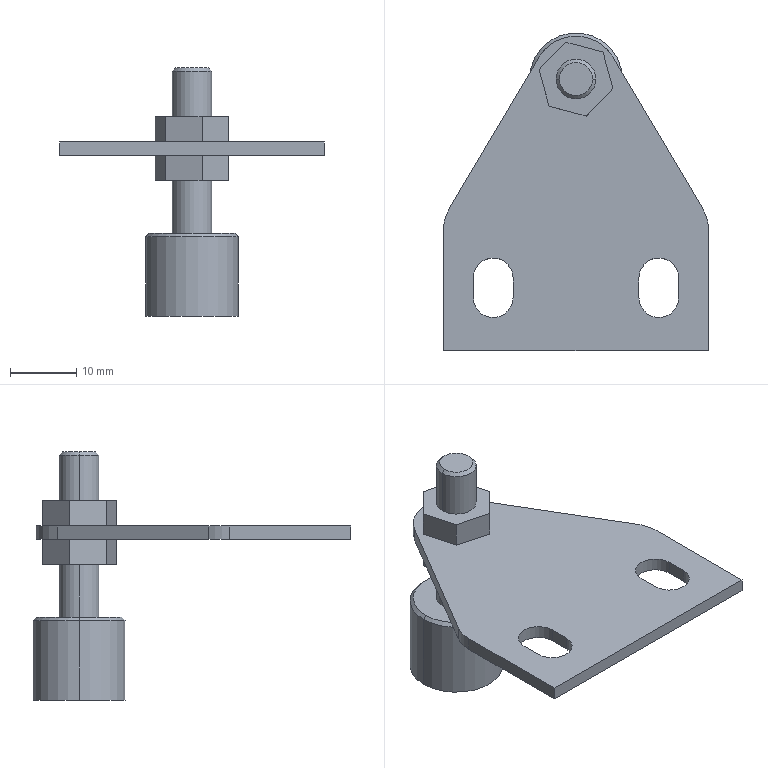Part | SolidWorks | features BaseBody 2 | 2 solids | 51 faces | box 40 x 48 x 37.5 mm | volume 5719 mm3 | plane 30 | cylinder 17 | cone 4 | commonest cylinder face diameters 6 x12 12 x2 14 x2 13 x1
STEP:
#1=CARTESIAN_POINT('',(-3.,41.,2.));
#2=VERTEX_POINT('',#1);
#3=CARTESIAN_POINT('',(3.,41.,2.));
#4=VERTEX_POINT('',#3);
#5=CARTESIAN_POINT('',(0.,41.,2.));
#6=DIRECTION('',(0.,0.,1.));
#7=DIRECTION('',(1.,0.,0.));
#8=AXIS2_PLACEMENT_3D('',#5,#6,#7);
#9=CIRCLE('',#8,3.);
#10=EDGE_CURVE('',#2,#4,#9,.T.);
#11=ORIENTED_EDGE('',*,*,#10,.T.);
#12=CARTESIAN_POINT('',(3.,41.,0.));
#13=VERTEX_POINT('',#12);
#14=CARTESIAN_POINT('',(3.,41.,2.));
#15=DIRECTION('',(0.,0.,-1.));
#16=VECTOR('',#15,1000.);
#17=LINE('',#14,#16);
#18=EDGE_CURVE('',#4,#13,#17,.T.);
#19=ORIENTED_EDGE('',*,*,#18,.T.);
#20=CARTESIAN_POINT('',(-3.,41.,0.));
#21=VERTEX_POINT('',#20);
#22=CARTESIAN_POINT('',(0.,41.,0.));
#23=DIRECTION('',(0.,0.,1.));
#24=DIRECTION('',(1.,0.,0.));
#25=AXIS2_PLACEMENT_3D('',#22,#23,#24);
#26=CIRCLE('',#25,3.);
#27=EDGE_CURVE('',#21,#13,#26,.T.);
#28=ORIENTED_EDGE('',*,*,#27,.F.);
#29=CARTESIAN_POINT('',(-3.,41.,2.));
#30=DIRECTION('',(0.,0.,-1.));
#31=VECTOR('',#30,1000.);
#32=LINE('',#29,#31);
#33=EDGE_CURVE('',#2,#21,#32,.T.);
#34=ORIENTED_EDGE('',*,*,#33,.F.);
#35=EDGE_LOOP('',(#11,#19,#28,#34));
#36=FACE_OUTER_BOUND('',#35,.T.);
#37=CARTESIAN_POINT('',(0.,41.,2.));
#38=DIRECTION('',(0.,0.,-1.));
#39=DIRECTION('',(-1.,0.,0.));
#40=AXIS2_PLACEMENT_3D('',#37,#38,#39);
#41=CYLINDRICAL_SURFACE('',#40,3.);
#42=ADVANCED_FACE('',(#36),#41,.F.);
#43=CARTESIAN_POINT('',(-9.5,11.,2.));
#44=VERTEX_POINT('',#43);
#45=CARTESIAN_POINT('',(-15.5,11.,2.));
#46=VERTEX_POINT('',#45);
#47=CARTESIAN_POINT('',(-12.5,11.,2.));
#48=DIRECTION('',(0.,0.,1.));
#49=DIRECTION('',(1.,0.,0.));
#50=AXIS2_PLACEMENT_3D('',#47,#48,#49);
#51=CIRCLE('',#50,3.);
#52=EDGE_CURVE('',#44,#46,#51,.T.);
#53=ORIENTED_EDGE('',*,*,#52,.F.);
#54=CARTESIAN_POINT('',(-9.5,8.,2.));
#55=VERTEX_POINT('',#54);
#56=CARTESIAN_POINT('',(-9.5,11.,2.));
#57=DIRECTION('',(0.,1.,0.));
#58=VECTOR('',#57,1000.);
#59=LINE('',#56,#58);
#60=EDGE_CURVE('',#55,#44,#59,.T.);
#61=ORIENTED_EDGE('',*,*,#60,.F.);
#62=CARTESIAN_POINT('',(-15.5,8.,2.));
#63=VERTEX_POINT('',#62);
#64=CARTESIAN_POINT('',(-12.5,8.,2.));
#65=DIRECTION('',(0.,0.,1.));
#66=DIRECTION('',(1.,0.,0.));
#67=AXIS2_PLACEMENT_3D('',#64,#65,#66);
#68=CIRCLE('',#67,3.);
#69=EDGE_CURVE('',#63,#55,#68,.T.);
#70=ORIENTED_EDGE('',*,*,#69,.F.);
#71=CARTESIAN_POINT('',(-15.5,11.,2.));
#72=DIRECTION('',(0.,-1.,0.));
#73=VECTOR('',#72,1000.);
#74=LINE('',#71,#73);
#75=EDGE_CURVE('',#46,#63,#74,.T.);
#76=ORIENTED_EDGE('',*,*,#75,.F.);
#77=EDGE_LOOP('',(#53,#61,#70,#76));
#78=FACE_BOUND('',#77,.T.);
#79=CARTESIAN_POINT('',(-20.,18.356,2.));
#80=VERTEX_POINT('',#79);
#81=CARTESIAN_POINT('',(-20.,0.,2.));
#82=VERTEX_POINT('',#81);
#83=CARTESIAN_POINT('',(-20.,0.,2.));
#84=DIRECTION('',(0.,-1.,0.));
#85=VECTOR('',#84,1000.);
#86=LINE('',#83,#85);
#87=EDGE_CURVE('',#80,#82,#86,.T.);
#88=ORIENTED_EDGE('',*,*,#87,.T.);
#89=CARTESIAN_POINT('',(20.,0.,2.));
#90=VERTEX_POINT('',#89);
#91=CARTESIAN_POINT('',(-20.,0.,2.));
#92=DIRECTION('',(1.,0.,0.));
#93=VECTOR('',#92,1000.);
#94=LINE('',#91,#93);
#95=EDGE_CURVE('',#82,#90,#94,.T.);
#96=ORIENTED_EDGE('',*,*,#95,.T.);
#97=CARTESIAN_POINT('',(20.,18.356,2.));
#98=VERTEX_POINT('',#97);
#99=CARTESIAN_POINT('',(20.,0.,2.));
#100=DIRECTION('',(0.,1.,0.));
#101=VECTOR('',#100,1000.);
#102=LINE('',#99,#101);
#103=EDGE_CURVE('',#90,#98,#102,.T.);
#104=ORIENTED_EDGE('',*,*,#103,.T.);
#105=CARTESIAN_POINT('',(19.162,21.415,2.));
#106=VERTEX_POINT('',#105);
#107=CARTESIAN_POINT('',(14.,18.356,2.));
#108=DIRECTION('',(0.,0.,1.));
#109=DIRECTION('',(-1.,0.,0.));
#110=AXIS2_PLACEMENT_3D('',#107,#108,#109);
#111=CIRCLE('',#110,6.);
#112=EDGE_CURVE('',#98,#106,#111,.T.);
#113=ORIENTED_EDGE('',*,*,#112,.T.);
#114=CARTESIAN_POINT('',(5.592,44.314,2.));
#115=VERTEX_POINT('',#114);
#116=CARTESIAN_POINT('',(19.162,21.415,2.));
#117=DIRECTION('',(-0.5098,0.8603,0.));
#118=VECTOR('',#117,1000.);
#119=LINE('',#116,#118);
#120=EDGE_CURVE('',#106,#115,#119,.T.);
#121=ORIENTED_EDGE('',*,*,#120,.T.);
#122=CARTESIAN_POINT('',(-5.592,44.314,2.));
#123=VERTEX_POINT('',#122);
#124=CARTESIAN_POINT('',(0.,41.,2.));
#125=DIRECTION('',(0.,0.,1.));
#126=DIRECTION('',(1.,0.,0.));
#127=AXIS2_PLACEMENT_3D('',#124,#125,#126);
#128=CIRCLE('',#127,6.5);
#129=EDGE_CURVE('',#115,#123,#128,.T.);
#130=ORIENTED_EDGE('',*,*,#129,.T.);
#131=CARTESIAN_POINT('',(-19.162,21.415,2.));
#132=VERTEX_POINT('',#131);
#133=CARTESIAN_POINT('',(-19.162,21.415,2.));
#134=DIRECTION('',(-0.5098,-0.8603,0.));
#135=VECTOR('',#134,1000.);
#136=LINE('',#133,#135);
#137=EDGE_CURVE('',#123,#132,#136,.T.);
#138=ORIENTED_EDGE('',*,*,#137,.T.);
#139=CARTESIAN_POINT('',(-14.,18.356,2.));
#140=DIRECTION('',(0.,0.,1.));
#141=DIRECTION('',(-1.,0.,0.));
#142=AXIS2_PLACEMENT_3D('',#139,#140,#141);
#143=CIRCLE('',#142,6.);
#144=EDGE_CURVE('',#132,#80,#143,.T.);
#145=ORIENTED_EDGE('',*,*,#144,.T.);
#146=EDGE_LOOP('',(#88,#96,#104,#113,#121,#130,#138,#145));
#147=FACE_OUTER_BOUND('',#146,.T.);
#148=ORIENTED_EDGE('',*,*,#10,.F.);
#149=CARTESIAN_POINT('',(0.,41.,2.));
#150=DIRECTION('',(0.,0.,1.));
#151=DIRECTION('',(1.,0.,0.));
#152=AXIS2_PLACEMENT_3D('',#149,#150,#151);
#153=CIRCLE('',#152,3.);
#154=EDGE_CURVE('',#4,#2,#153,.T.);
#155=ORIENTED_EDGE('',*,*,#154,.F.);
#156=EDGE_LOOP('',(#148,#155));
#157=FACE_BOUND('',#156,.T.);
#158=CARTESIAN_POINT('',(15.5,11.,2.));
#159=VERTEX_POINT('',#158);
#160=CARTESIAN_POINT('',(9.5,11.,2.));
#161=VERTEX_POINT('',#160);
#162=CARTESIAN_POINT('',(12.5,11.,2.));
#163=DIRECTION('',(0.,0.,1.));
#164=DIRECTION('',(1.,0.,0.));
#165=AXIS2_PLACEMENT_3D('',#162,#163,#164);
#166=CIRCLE('',#165,3.);
#167=EDGE_CURVE('',#159,#161,#166,.T.);
#168=ORIENTED_EDGE('',*,*,#167,.F.);
#169=CARTESIAN_POINT('',(15.5,8.,2.));
#170=VERTEX_POINT('',#169);
#171=CARTESIAN_POINT('',(15.5,11.,2.));
#172=DIRECTION('',(0.,1.,0.));
#173=VECTOR('',#172,1000.);
#174=LINE('',#171,#173);
#175=EDGE_CURVE('',#170,#159,#174,.T.);
#176=ORIENTED_EDGE('',*,*,#175,.F.);
#177=CARTESIAN_POINT('',(9.5,8.,2.));
#178=VERTEX_POINT('',#177);
#179=CARTESIAN_POINT('',(12.5,8.,2.));
#180=DIRECTION('',(0.,0.,1.));
#181=DIRECTION('',(1.,0.,0.));
#182=AXIS2_PLACEMENT_3D('',#179,#180,#181);
#183=CIRCLE('',#182,3.);
#184=EDGE_CURVE('',#178,#170,#183,.T.);
#185=ORIENTED_EDGE('',*,*,#184,.F.);
#186=CARTESIAN_POINT('',(9.5,11.,2.));
#187=DIRECTION('',(0.,-1.,0.));
#188=VECTOR('',#187,1000.);
#189=LINE('',#186,#188);
#190=EDGE_CURVE('',#161,#178,#189,.T.);
#191=ORIENTED_EDGE('',*,*,#190,.F.);
#192=EDGE_LOOP('',(#168,#176,#185,#191));
#193=FACE_BOUND('',#192,.T.);
#194=CARTESIAN_POINT('',(-14.,18.356,2.));
#195=DIRECTION('',(0.,0.,-1.));
#196=DIRECTION('',(-1.,0.,0.));
#197=AXIS2_PLACEMENT_3D('',#194,#195,#196);
#198=PLANE('',#197);
#199=ADVANCED_FACE('',(#78,#147,#157,#193),#198,.F.);
#200=CARTESIAN_POINT('',(-9.5,8.,0.));
#201=VERTEX_POINT('',#200);
#202=CARTESIAN_POINT('',(-9.5,11.,0.));
#203=VERTEX_POINT('',#202);
#204=CARTESIAN_POINT('',(-9.5,11.,0.));
#205=DIRECTION('',(0.,1.,0.));
#206=VECTOR('',#205,1000.);
#207=LINE('',#204,#206);
#208=EDGE_CURVE('',#201,#203,#207,.T.);
#209=ORIENTED_EDGE('',*,*,#208,.T.);
#210=CARTESIAN_POINT('',(-15.5,11.,0.));
#211=VERTEX_POINT('',#210);
#212=CARTESIAN_POINT('',(-12.5,11.,0.));
#213=DIRECTION('',(0.,0.,1.));
#214=DIRECTION('',(1.,0.,0.));
#215=AXIS2_PLACEMENT_3D('',#212,#213,#214);
#216=CIRCLE('',#215,3.);
#217=EDGE_CURVE('',#203,#211,#216,.T.);
#218=ORIENTED_EDGE('',*,*,#217,.T.);
#219=CARTESIAN_POINT('',(-15.5,8.,0.));
#220=VERTEX_POINT('',#219);
#221=CARTESIAN_POINT('',(-15.5,11.,0.));
#222=DIRECTION('',(0.,-1.,0.));
#223=VECTOR('',#222,1000.);
#224=LINE('',#221,#223);
#225=EDGE_CURVE('',#211,#220,#224,.T.);
#226=ORIENTED_EDGE('',*,*,#225,.T.);
#227=CARTESIAN_POINT('',(-12.5,8.,0.));
#228=DIRECTION('',(0.,0.,1.));
#229=DIRECTION('',(1.,0.,0.));
#230=AXIS2_PLACEMENT_3D('',#227,#228,#229);
#231=CIRCLE('',#230,3.);
#232=EDGE_CURVE('',#220,#201,#231,.T.);
#233=ORIENTED_EDGE('',*,*,#232,.T.);
#234=EDGE_LOOP('',(#209,#218,#226,#233));
#235=FACE_BOUND('',#234,.T.);
#236=CARTESIAN_POINT('',(-20.,18.356,0.));
#237=VERTEX_POINT('',#236);
#238=CARTESIAN_POINT('',(-20.,0.,0.));
#239=VERTEX_POINT('',#238);
#240=CARTESIAN_POINT('',(-20.,0.,0.));
#241=DIRECTION('',(0.,-1.,0.));
#242=VECTOR('',#241,1000.);
#243=LINE('',#240,#242);
#244=EDGE_CURVE('',#237,#239,#243,.T.);
#245=ORIENTED_EDGE('',*,*,#244,.F.);
#246=CARTESIAN_POINT('',(-19.162,21.415,0.));
#247=VERTEX_POINT('',#246);
#248=CARTESIAN_POINT('',(-14.,18.356,0.));
#249=DIRECTION('',(0.,0.,1.));
#250=DIRECTION('',(-1.,0.,0.));
#251=AXIS2_PLACEMENT_3D('',#248,#249,#250);
#252=CIRCLE('',#251,6.);
#253=EDGE_CURVE('',#247,#237,#252,.T.);
#254=ORIENTED_EDGE('',*,*,#253,.F.);
#255=CARTESIAN_POINT('',(-5.592,44.314,0.));
#256=VERTEX_POINT('',#255);
#257=CARTESIAN_POINT('',(-19.162,21.415,0.));
#258=DIRECTION('',(-0.5098,-0.8603,0.));
#259=VECTOR('',#258,1000.);
#260=LINE('',#257,#259);
#261=EDGE_CURVE('',#256,#247,#260,.T.);
#262=ORIENTED_EDGE('',*,*,#261,.F.);
#263=CARTESIAN_POINT('',(5.592,44.314,0.));
#264=VERTEX_POINT('',#263);
#265=CARTESIAN_POINT('',(0.,41.,0.));
#266=DIRECTION('',(0.,0.,1.));
#267=DIRECTION('',(1.,0.,0.));
#268=AXIS2_PLACEMENT_3D('',#265,#266,#267);
#269=CIRCLE('',#268,6.5);
#270=EDGE_CURVE('',#264,#256,#269,.T.);
#271=ORIENTED_EDGE('',*,*,#270,.F.);
#272=CARTESIAN_POINT('',(19.162,21.415,0.));
#273=VERTEX_POINT('',#272);
#274=CARTESIAN_POINT('',(19.162,21.415,0.));
#275=DIRECTION('',(-0.5098,0.8603,0.));
#276=VECTOR('',#275,1000.);
#277=LINE('',#274,#276);
#278=EDGE_CURVE('',#273,#264,#277,.T.);
#279=ORIENTED_EDGE('',*,*,#278,.F.);
#280=CARTESIAN_POINT('',(20.,18.356,0.));
#281=VERTEX_POINT('',#280);
#282=CARTESIAN_POINT('',(14.,18.356,0.));
#283=DIRECTION('',(0.,0.,1.));
#284=DIRECTION('',(-1.,0.,0.));
#285=AXIS2_PLACEMENT_3D('',#282,#283,#284);
#286=CIRCLE('',#285,6.);
#287=EDGE_CURVE('',#281,#273,#286,.T.);
#288=ORIENTED_EDGE('',*,*,#287,.F.);
#289=CARTESIAN_POINT('',(20.,0.,0.));
#290=VERTEX_POINT('',#289);
#291=CARTESIAN_POINT('',(20.,0.,0.));
#292=DIRECTION('',(0.,1.,0.));
#293=VECTOR('',#292,1000.);
#294=LINE('',#291,#293);
#295=EDGE_CURVE('',#290,#281,#294,.T.);
#296=ORIENTED_EDGE('',*,*,#295,.F.);
#297=CARTESIAN_POINT('',(-20.,0.,0.));
#298=DIRECTION('',(1.,0.,0.));
#299=VECTOR('',#298,1000.);
#300=LINE('',#297,#299);
#301=EDGE_CURVE('',#239,#290,#300,.T.);
#302=ORIENTED_EDGE('',*,*,#301,.F.);
#303=EDGE_LOOP('',(#245,#254,#262,#271,#279,#288,#296,#302));
#304=FACE_OUTER_BOUND('',#303,.T.);
#305=ORIENTED_EDGE('',*,*,#27,.T.);
#306=CARTESIAN_POINT('',(0.,41.,0.));
#307=DIRECTION('',(0.,0.,1.));
#308=DIRECTION('',(1.,0.,0.));
#309=AXIS2_PLACEMENT_3D('',#306,#307,#308);
#310=CIRCLE('',#309,3.);
#311=EDGE_CURVE('',#13,#21,#310,.T.);
#312=ORIENTED_EDGE('',*,*,#311,.T.);
#313=EDGE_LOOP('',(#305,#312));
#314=FACE_BOUND('',#313,.T.);
#315=CARTESIAN_POINT('',(15.5,8.,0.));
#316=VERTEX_POINT('',#315);
#317=CARTESIAN_POINT('',(15.5,11.,0.));
#318=VERTEX_POINT('',#317);
#319=CARTESIAN_POINT('',(15.5,11.,0.));
#320=DIRECTION('',(0.,1.,0.));
#321=VECTOR('',#320,1000.);
#322=LINE('',#319,#321);
#323=EDGE_CURVE('',#316,#318,#322,.T.);
#324=ORIENTED_EDGE('',*,*,#323,.T.);
#325=CARTESIAN_POINT('',(9.5,11.,0.));
#326=VERTEX_POINT('',#325);
#327=CARTESIAN_POINT('',(12.5,11.,0.));
#328=DIRECTION('',(0.,0.,1.));
#329=DIRECTION('',(1.,0.,0.));
#330=AXIS2_PLACEMENT_3D('',#327,#328,#329);
#331=CIRCLE('',#330,3.);
#332=EDGE_CURVE('',#318,#326,#331,.T.);
#333=ORIENTED_EDGE('',*,*,#332,.T.);
#334=CARTESIAN_POINT('',(9.5,8.,0.));
#335=VERTEX_POINT('',#334);
#336=CARTESIAN_POINT('',(9.5,11.,0.));
#337=DIRECTION('',(0.,-1.,0.));
#338=VECTOR('',#337,1000.);
#339=LINE('',#336,#338);
#340=EDGE_CURVE('',#326,#335,#339,.T.);
#341=ORIENTED_EDGE('',*,*,#340,.T.);
#342=CARTESIAN_POINT('',(12.5,8.,0.));
#343=DIRECTION('',(0.,0.,1.));
#344=DIRECTION('',(1.,0.,0.));
#345=AXIS2_PLACEMENT_3D('',#342,#343,#344);
#346=CIRCLE('',#345,3.);
#347=EDGE_CURVE('',#335,#316,#346,.T.);
#348=ORIENTED_EDGE('',*,*,#347,.T.);
#349=EDGE_LOOP('',(#324,#333,#341,#348));
#350=FACE_BOUND('',#349,.T.);
#351=CARTESIAN_POINT('',(-14.,18.356,0.));
#352=DIRECTION('',(0.,0.,-1.));
#353=DIRECTION('',(-1.,0.,0.));
#354=AXIS2_PLACEMENT_3D('',#351,#352,#353);
#355=PLANE('',#354);
#356=ADVANCED_FACE('',(#235,#304,#314,#350),#355,.T.);
#357=ORIENTED_EDGE('',*,*,#244,.T.);
#358=CARTESIAN_POINT('',(-20.,0.,2.));
#359=DIRECTION('',(0.,0.,-1.));
#360=VECTOR('',#359,1000.);
#361=LINE('',#358,#360);
#362=EDGE_CURVE('',#82,#239,#361,.T.);
#363=ORIENTED_EDGE('',*,*,#362,.F.);
#364=ORIENTED_EDGE('',*,*,#87,.F.);
#365=CARTESIAN_POINT('',(-20.,18.356,2.));
#366=DIRECTION('',(0.,0.,-1.));
#367=VECTOR('',#366,1000.);
#368=LINE('',#365,#367);
#369=EDGE_CURVE('',#80,#237,#368,.T.);
#370=ORIENTED_EDGE('',*,*,#369,.T.);
#371=EDGE_LOOP('',(#357,#363,#364,#370));
#372=FACE_OUTER_BOUND('',#371,.T.);
#373=CARTESIAN_POINT('',(-20.,0.,2.));
#374=DIRECTION('',(1.,0.,0.));
#375=DIRECTION('',(0.,0.,-1.));
#376=AXIS2_PLACEMENT_3D('',#373,#374,#375);
#377=PLANE('',#376);
#378=ADVANCED_FACE('',(#372),#377,.F.);
#379=ORIENTED_EDGE('',*,*,#301,.T.);
#380=CARTESIAN_POINT('',(20.,0.,2.));
#381=DIRECTION('',(0.,0.,-1.));
#382=VECTOR('',#381,1000.);
#383=LINE('',#380,#382);
#384=EDGE_CURVE('',#90,#290,#383,.T.);
#385=ORIENTED_EDGE('',*,*,#384,.F.);
#386=ORIENTED_EDGE('',*,*,#95,.F.);
#387=ORIENTED_EDGE('',*,*,#362,.T.);
#388=EDGE_LOOP('',(#379,#385,#386,#387));
#389=FACE_OUTER_BOUND('',#388,.T.);
#390=CARTESIAN_POINT('',(-20.,0.,2.));
#391=DIRECTION('',(0.,1.,0.));
#392=DIRECTION('',(0.,0.,1.));
#393=AXIS2_PLACEMENT_3D('',#390,#391,#392);
#394=PLANE('',#393);
#395=ADVANCED_FACE('',(#389),#394,.F.);
#396=ORIENTED_EDGE('',*,*,#295,.T.);
#397=CARTESIAN_POINT('',(20.,18.356,2.));
#398=DIRECTION('',(0.,0.,-1.));
#399=VECTOR('',#398,1000.);
#400=LINE('',#397,#399);
#401=EDGE_CURVE('',#98,#281,#400,.T.);
#402=ORIENTED_EDGE('',*,*,#401,.F.);
#403=ORIENTED_EDGE('',*,*,#103,.F.);
#404=ORIENTED_EDGE('',*,*,#384,.T.);
#405=EDGE_LOOP('',(#396,#402,#403,#404));
#406=FACE_OUTER_BOUND('',#405,.T.);
#407=CARTESIAN_POINT('',(20.,0.,2.));
#408=DIRECTION('',(-1.,0.,0.));
#409=DIRECTION('',(0.,0.,1.));
#410=AXIS2_PLACEMENT_3D('',#407,#408,#409);
#411=PLANE('',#410);
#412=ADVANCED_FACE('',(#406),#411,.F.);
#413=ORIENTED_EDGE('',*,*,#287,.T.);
#414=CARTESIAN_POINT('',(19.162,21.415,2.));
#415=DIRECTION('',(0.,0.,-1.));
#416=VECTOR('',#415,1000.);
#417=LINE('',#414,#416);
#418=EDGE_CURVE('',#106,#273,#417,.T.);
#419=ORIENTED_EDGE('',*,*,#418,.F.);
#420=ORIENTED_EDGE('',*,*,#112,.F.);
#421=ORIENTED_EDGE('',*,*,#401,.T.);
#422=EDGE_LOOP('',(#413,#419,#420,#421));
#423=FACE_OUTER_BOUND('',#422,.T.);
#424=CARTESIAN_POINT('',(14.,18.356,2.));
#425=DIRECTION('',(0.,0.,-1.));
#426=DIRECTION('',(-1.,0.,0.));
#427=AXIS2_PLACEMENT_3D('',#424,#425,#426);
#428=CYLINDRICAL_SURFACE('',#427,6.);
#429=ADVANCED_FACE('',(#423),#428,.T.);
#430=ORIENTED_EDGE('',*,*,#278,.T.);
#431=CARTESIAN_POINT('',(5.592,44.314,2.));
#432=DIRECTION('',(0.,0.,-1.));
#433=VECTOR('',#432,1000.);
#434=LINE('',#431,#433);
#435=EDGE_CURVE('',#115,#264,#434,.T.);
#436=ORIENTED_EDGE('',*,*,#435,.F.);
#437=ORIENTED_EDGE('',*,*,#120,.F.);
#438=ORIENTED_EDGE('',*,*,#418,.T.);
#439=EDGE_LOOP('',(#430,#436,#437,#438));
#440=FACE_OUTER_BOUND('',#439,.T.);
#441=CARTESIAN_POINT('',(19.162,21.415,2.));
#442=DIRECTION('',(-0.8603,-0.5098,0.));
#443=DIRECTION('',(0.5098,-0.8603,0.));
#444=AXIS2_PLACEMENT_3D('',#441,#442,#443);
#445=PLANE('',#444);
#446=ADVANCED_FACE('',(#440),#445,.F.);
#447=ORIENTED_EDGE('',*,*,#270,.T.);
#448=CARTESIAN_POINT('',(-5.592,44.314,2.));
#449=DIRECTION('',(0.,0.,-1.));
#450=VECTOR('',#449,1000.);
#451=LINE('',#448,#450);
#452=EDGE_CURVE('',#123,#256,#451,.T.);
#453=ORIENTED_EDGE('',*,*,#452,.F.);
#454=ORIENTED_EDGE('',*,*,#129,.F.);
#455=ORIENTED_EDGE('',*,*,#435,.T.);
#456=EDGE_LOOP('',(#447,#453,#454,#455));
#457=FACE_OUTER_BOUND('',#456,.T.);
#458=CARTESIAN_POINT('',(0.,41.,2.));
#459=DIRECTION('',(0.,0.,-1.));
#460=DIRECTION('',(-1.,0.,0.));
#461=AXIS2_PLACEMENT_3D('',#458,#459,#460);
#462=CYLINDRICAL_SURFACE('',#461,6.5);
#463=ADVANCED_FACE('',(#457),#462,.T.);
#464=ORIENTED_EDGE('',*,*,#261,.T.);
#465=CARTESIAN_POINT('',(-19.162,21.415,2.));
#466=DIRECTION('',(0.,0.,-1.));
#467=VECTOR('',#466,1000.);
#468=LINE('',#465,#467);
#469=EDGE_CURVE('',#132,#247,#468,.T.);
#470=ORIENTED_EDGE('',*,*,#469,.F.);
#471=ORIENTED_EDGE('',*,*,#137,.F.);
#472=ORIENTED_EDGE('',*,*,#452,.T.);
#473=EDGE_LOOP('',(#464,#470,#471,#472));
#474=FACE_OUTER_BOUND('',#473,.T.);
#475=CARTESIAN_POINT('',(-19.162,21.415,2.));
#476=DIRECTION('',(0.8603,-0.5098,0.));
#477=DIRECTION('',(0.5098,0.8603,0.));
#478=AXIS2_PLACEMENT_3D('',#475,#476,#477);
#479=PLANE('',#478);
#480=ADVANCED_FACE('',(#474),#479,.F.);
#481=ORIENTED_EDGE('',*,*,#253,.T.);
#482=ORIENTED_EDGE('',*,*,#369,.F.);
#483=ORIENTED_EDGE('',*,*,#144,.F.);
#484=ORIENTED_EDGE('',*,*,#469,.T.);
#485=EDGE_LOOP('',(#481,#482,#483,#484));
#486=FACE_OUTER_BOUND('',#485,.T.);
#487=CARTESIAN_POINT('',(-14.,18.356,2.));
#488=DIRECTION('',(0.,0.,-1.));
#489=DIRECTION('',(-1.,0.,0.));
#490=AXIS2_PLACEMENT_3D('',#487,#488,#489);
#491=CYLINDRICAL_SURFACE('',#490,6.);
#492=ADVANCED_FACE('',(#486),#491,.T.);
#493=ORIENTED_EDGE('',*,*,#18,.F.);
#494=ORIENTED_EDGE('',*,*,#154,.T.);
#495=ORIENTED_EDGE('',*,*,#33,.T.);
#496=ORIENTED_EDGE('',*,*,#311,.F.);
#497=EDGE_LOOP('',(#493,#494,#495,#496));
#498=FACE_OUTER_BOUND('',#497,.T.);
#499=CARTESIAN_POINT('',(0.,41.,2.));
#500=DIRECTION('',(0.,0.,-1.));
#501=DIRECTION('',(-1.,0.,0.));
#502=AXIS2_PLACEMENT_3D('',#499,#500,#501);
#503=CYLINDRICAL_SURFACE('',#502,3.);
#504=ADVANCED_FACE('',(#498),#503,.F.);
#505=ORIENTED_EDGE('',*,*,#217,.F.);
#506=CARTESIAN_POINT('',(-9.5,11.,2.));
#507=DIRECTION('',(0.,0.,-1.));
#508=VECTOR('',#507,1000.);
#509=LINE('',#506,#508);
#510=EDGE_CURVE('',#44,#203,#509,.T.);
#511=ORIENTED_EDGE('',*,*,#510,.F.);
#512=ORIENTED_EDGE('',*,*,#52,.T.);
#513=CARTESIAN_POINT('',(-15.5,11.,2.));
#514=DIRECTION('',(0.,0.,-1.));
#515=VECTOR('',#514,1000.);
#516=LINE('',#513,#515);
#517=EDGE_CURVE('',#46,#211,#516,.T.);
#518=ORIENTED_EDGE('',*,*,#517,.T.);
#519=EDGE_LOOP('',(#505,#511,#512,#518));
#520=FACE_OUTER_BOUND('',#519,.T.);
#521=CARTESIAN_POINT('',(-12.5,11.,2.));
#522=DIRECTION('',(0.,0.,-1.));
#523=DIRECTION('',(-1.,0.,0.));
#524=AXIS2_PLACEMENT_3D('',#521,#522,#523);
#525=CYLINDRICAL_SURFACE('',#524,3.);
#526=ADVANCED_FACE('',(#520),#525,.F.);
#527=ORIENTED_EDGE('',*,*,#225,.F.);
#528=ORIENTED_EDGE('',*,*,#517,.F.);
#529=ORIENTED_EDGE('',*,*,#75,.T.);
#530=CARTESIAN_POINT('',(-15.5,8.,2.));
#531=DIRECTION('',(0.,0.,-1.));
#532=VECTOR('',#531,1000.);
#533=LINE('',#530,#532);
#534=EDGE_CURVE('',#63,#220,#533,.T.);
#535=ORIENTED_EDGE('',*,*,#534,.T.);
#536=EDGE_LOOP('',(#527,#528,#529,#535));
#537=FACE_OUTER_BOUND('',#536,.T.);
#538=CARTESIAN_POINT('',(-15.5,11.,2.));
#539=DIRECTION('',(1.,0.,0.));
#540=DIRECTION('',(0.,0.,-1.));
#541=AXIS2_PLACEMENT_3D('',#538,#539,#540);
#542=PLANE('',#541);
#543=ADVANCED_FACE('',(#537),#542,.T.);
#544=ORIENTED_EDGE('',*,*,#232,.F.);
#545=ORIENTED_EDGE('',*,*,#534,.F.);
#546=ORIENTED_EDGE('',*,*,#69,.T.);
#547=CARTESIAN_POINT('',(-9.5,8.,2.));
#548=DIRECTION('',(0.,0.,-1.));
#549=VECTOR('',#548,1000.);
#550=LINE('',#547,#549);
#551=EDGE_CURVE('',#55,#201,#550,.T.);
#552=ORIENTED_EDGE('',*,*,#551,.T.);
#553=EDGE_LOOP('',(#544,#545,#546,#552));
#554=FACE_OUTER_BOUND('',#553,.T.);
#555=CARTESIAN_POINT('',(-12.5,8.,2.));
#556=DIRECTION('',(0.,0.,-1.));
#557=DIRECTION('',(-1.,0.,0.));
#558=AXIS2_PLACEMENT_3D('',#555,#556,#557);
#559=CYLINDRICAL_SURFACE('',#558,3.);
#560=ADVANCED_FACE('',(#554),#559,.F.);
#561=ORIENTED_EDGE('',*,*,#208,.F.);
#562=ORIENTED_EDGE('',*,*,#551,.F.);
#563=ORIENTED_EDGE('',*,*,#60,.T.);
#564=ORIENTED_EDGE('',*,*,#510,.T.);
#565=EDGE_LOOP('',(#561,#562,#563,#564));
#566=FACE_OUTER_BOUND('',#565,.T.);
#567=CARTESIAN_POINT('',(-9.5,11.,2.));
#568=DIRECTION('',(-1.,0.,0.));
#569=DIRECTION('',(0.,0.,1.));
#570=AXIS2_PLACEMENT_3D('',#567,#568,#569);
#571=PLANE('',#570);
#572=ADVANCED_FACE('',(#566),#571,.T.);
#573=ORIENTED_EDGE('',*,*,#332,.F.);
#574=CARTESIAN_POINT('',(15.5,11.,2.));
#575=DIRECTION('',(0.,0.,-1.));
#576=VECTOR('',#575,1000.);
#577=LINE('',#574,#576);
#578=EDGE_CURVE('',#159,#318,#577,.T.);
#579=ORIENTED_EDGE('',*,*,#578,.F.);
#580=ORIENTED_EDGE('',*,*,#167,.T.);
#581=CARTESIAN_POINT('',(9.5,11.,2.));
#582=DIRECTION('',(0.,0.,-1.));
#583=VECTOR('',#582,1000.);
#584=LINE('',#581,#583);
#585=EDGE_CURVE('',#161,#326,#584,.T.);
#586=ORIENTED_EDGE('',*,*,#585,.T.);
#587=EDGE_LOOP('',(#573,#579,#580,#586));
#588=FACE_OUTER_BOUND('',#587,.T.);
#589=CARTESIAN_POINT('',(12.5,11.,2.));
#590=DIRECTION('',(0.,0.,-1.));
#591=DIRECTION('',(-1.,0.,0.));
#592=AXIS2_PLACEMENT_3D('',#589,#590,#591);
#593=CYLINDRICAL_SURFACE('',#592,3.);
#594=ADVANCED_FACE('',(#588),#593,.F.);
#595=ORIENTED_EDGE('',*,*,#340,.F.);
#596=ORIENTED_EDGE('',*,*,#585,.F.);
#597=ORIENTED_EDGE('',*,*,#190,.T.);
#598=CARTESIAN_POINT('',(9.5,8.,2.));
#599=DIRECTION('',(0.,0.,-1.));
#600=VECTOR('',#599,1000.);
#601=LINE('',#598,#600);
#602=EDGE_CURVE('',#178,#335,#601,.T.);
#603=ORIENTED_EDGE('',*,*,#602,.T.);
#604=EDGE_LOOP('',(#595,#596,#597,#603));
#605=FACE_OUTER_BOUND('',#604,.T.);
#606=CARTESIAN_POINT('',(9.5,11.,2.));
#607=DIRECTION('',(1.,0.,0.));
#608=DIRECTION('',(0.,0.,-1.));
#609=AXIS2_PLACEMENT_3D('',#606,#607,#608);
#610=PLANE('',#609);
#611=ADVANCED_FACE('',(#605),#610,.T.);
#612=ORIENTED_EDGE('',*,*,#347,.F.);
#613=ORIENTED_EDGE('',*,*,#602,.F.);
#614=ORIENTED_EDGE('',*,*,#184,.T.);
#615=CARTESIAN_POINT('',(15.5,8.,2.));
#616=DIRECTION('',(0.,0.,-1.));
#617=VECTOR('',#616,1000.);
#618=LINE('',#615,#617);
#619=EDGE_CURVE('',#170,#316,#618,.T.);
#620=ORIENTED_EDGE('',*,*,#619,.T.);
#621=EDGE_LOOP('',(#612,#613,#614,#620));
#622=FACE_OUTER_BOUND('',#621,.T.);
#623=CARTESIAN_POINT('',(12.5,8.,2.));
#624=DIRECTION('',(0.,0.,-1.));
#625=DIRECTION('',(-1.,0.,0.));
#626=AXIS2_PLACEMENT_3D('',#623,#624,#625);
#627=CYLINDRICAL_SURFACE('',#626,3.);
#628=ADVANCED_FACE('',(#622),#627,.F.);
#629=ORIENTED_EDGE('',*,*,#323,.F.);
#630=ORIENTED_EDGE('',*,*,#619,.F.);
#631=ORIENTED_EDGE('',*,*,#175,.T.);
#632=ORIENTED_EDGE('',*,*,#578,.T.);
#633=EDGE_LOOP('',(#629,#630,#631,#632));
#634=FACE_OUTER_BOUND('',#633,.T.);
#635=CARTESIAN_POINT('',(15.5,11.,2.));
#636=DIRECTION('',(-1.,0.,0.));
#637=DIRECTION('',(0.,0.,1.));
#638=AXIS2_PLACEMENT_3D('',#635,#636,#637);
#639=PLANE('',#638);
#640=ADVANCED_FACE('',(#634),#639,.T.);
#641=CLOSED_SHELL('',(#42,#199,#356,#378,#395,#412,#429,#446,#463,#480,#492,#504,#526,#543,#560,#572,#594,#611,#628,#640));
#642=MANIFOLD_SOLID_BREP('',#641);
#643=CARTESIAN_POINT('',(6.5,41.,-11.8));
#644=VERTEX_POINT('',#643);
#645=CARTESIAN_POINT('',(-6.5,41.,-11.8));
#646=VERTEX_POINT('',#645);
#647=CARTESIAN_POINT('',(0.,41.,-11.8));
#648=DIRECTION('',(0.,0.,1.));
#649=DIRECTION('',(1.,0.,0.));
#650=AXIS2_PLACEMENT_3D('',#647,#648,#649);
#651=CIRCLE('',#650,6.5);
#652=EDGE_CURVE('',#644,#646,#651,.T.);
#653=ORIENTED_EDGE('',*,*,#652,.F.);
#654=CARTESIAN_POINT('',(7.,41.,-12.3));
#655=VERTEX_POINT('',#654);
#656=CARTESIAN_POINT('',(6.5,41.,-11.8));
#657=DIRECTION('',(0.7071,0.,-0.7071));
#658=VECTOR('',#657,1000.);
#659=LINE('',#656,#658);
#660=EDGE_CURVE('',#644,#655,#659,.T.);
#661=ORIENTED_EDGE('',*,*,#660,.T.);
#662=CARTESIAN_POINT('',(-7.,41.,-12.3));
#663=VERTEX_POINT('',#662);
#664=CARTESIAN_POINT('',(0.,41.,-12.3));
#665=DIRECTION('',(0.,0.,-1.));
#666=DIRECTION('',(1.,0.,0.));
#667=AXIS2_PLACEMENT_3D('',#664,#665,#666);
#668=CIRCLE('',#667,7.);
#669=EDGE_CURVE('',#663,#655,#668,.T.);
#670=ORIENTED_EDGE('',*,*,#669,.F.);
#671=CARTESIAN_POINT('',(-6.5,41.,-11.8));
#672=DIRECTION('',(-0.7071,0.,-0.7071));
#673=VECTOR('',#672,1000.);
#674=LINE('',#671,#673);
#675=EDGE_CURVE('',#646,#663,#674,.T.);
#676=ORIENTED_EDGE('',*,*,#675,.F.);
#677=EDGE_LOOP('',(#653,#661,#670,#676));
#678=FACE_OUTER_BOUND('',#677,.T.);
#679=CARTESIAN_POINT('',(0.,41.,-11.8));
#680=DIRECTION('',(0.,0.,-1.));
#681=DIRECTION('',(-1.,0.,0.));
#682=AXIS2_PLACEMENT_3D('',#679,#680,#681);
#683=CONICAL_SURFACE('',#682,6.5,0.7854);
#684=ADVANCED_FACE('',(#678),#683,.T.);
#685=CARTESIAN_POINT('',(2.5,41.,13.2));
#686=VERTEX_POINT('',#685);
#687=CARTESIAN_POINT('',(-2.5,41.,13.2));
#688=VERTEX_POINT('',#687);
#689=CARTESIAN_POINT('',(0.,41.,13.2));
#690=DIRECTION('',(0.,0.,1.));
#691=DIRECTION('',(1.,0.,0.));
#692=AXIS2_PLACEMENT_3D('',#689,#690,#691);
#693=CIRCLE('',#692,2.5);
#694=EDGE_CURVE('',#686,#688,#693,.T.);
#695=ORIENTED_EDGE('',*,*,#694,.F.);
#696=CARTESIAN_POINT('',(3.,41.,12.7));
#697=VERTEX_POINT('',#696);
#698=CARTESIAN_POINT('',(2.5,41.,13.2));
#699=DIRECTION('',(0.7071,0.,-0.7071));
#700=VECTOR('',#699,1000.);
#701=LINE('',#698,#700);
#702=EDGE_CURVE('',#686,#697,#701,.T.);
#703=ORIENTED_EDGE('',*,*,#702,.T.);
#704=CARTESIAN_POINT('',(-3.,41.,12.7));
#705=VERTEX_POINT('',#704);
#706=CARTESIAN_POINT('',(0.,41.,12.7));
#707=DIRECTION('',(0.,0.,-1.));
#708=DIRECTION('',(1.,0.,0.));
#709=AXIS2_PLACEMENT_3D('',#706,#707,#708);
#710=CIRCLE('',#709,3.);
#711=EDGE_CURVE('',#705,#697,#710,.T.);
#712=ORIENTED_EDGE('',*,*,#711,.F.);
#713=CARTESIAN_POINT('',(-2.5,41.,13.2));
#714=DIRECTION('',(-0.7071,0.,-0.7071));
#715=VECTOR('',#714,1000.);
#716=LINE('',#713,#715);
#717=EDGE_CURVE('',#688,#705,#716,.T.);
#718=ORIENTED_EDGE('',*,*,#717,.F.);
#719=EDGE_LOOP('',(#695,#703,#712,#718));
#720=FACE_OUTER_BOUND('',#719,.T.);
#721=CARTESIAN_POINT('',(0.,41.,13.2));
#722=DIRECTION('',(0.,0.,-1.));
#723=DIRECTION('',(-1.,0.,0.));
#724=AXIS2_PLACEMENT_3D('',#721,#722,#723);
#725=CONICAL_SURFACE('',#724,2.5,0.7854);
#726=ADVANCED_FACE('',(#720),#725,.T.);
#727=ORIENTED_EDGE('',*,*,#711,.T.);
#728=CARTESIAN_POINT('',(3.,41.,5.8));
#729=VERTEX_POINT('',#728);
#730=CARTESIAN_POINT('',(3.,41.,13.2));
#731=DIRECTION('',(0.,0.,-1.));
#732=VECTOR('',#731,1000.);
#733=LINE('',#730,#732);
#734=EDGE_CURVE('',#697,#729,#733,.T.);
#735=ORIENTED_EDGE('',*,*,#734,.T.);
#736=CARTESIAN_POINT('',(-3.,41.,5.8));
#737=VERTEX_POINT('',#736);
#738=CARTESIAN_POINT('',(0.,41.,5.8));
#739=DIRECTION('',(0.,0.,1.));
#740=DIRECTION('',(1.,0.,0.));
#741=AXIS2_PLACEMENT_3D('',#738,#739,#740);
#742=CIRCLE('',#741,3.);
#743=EDGE_CURVE('',#729,#737,#742,.T.);
#744=ORIENTED_EDGE('',*,*,#743,.T.);
#745=CARTESIAN_POINT('',(-3.,41.,13.2));
#746=DIRECTION('',(0.,0.,-1.));
#747=VECTOR('',#746,1000.);
#748=LINE('',#745,#747);
#749=EDGE_CURVE('',#705,#737,#748,.T.);
#750=ORIENTED_EDGE('',*,*,#749,.F.);
#751=EDGE_LOOP('',(#727,#735,#744,#750));
#752=FACE_OUTER_BOUND('',#751,.T.);
#753=CARTESIAN_POINT('',(0.,41.,13.2));
#754=DIRECTION('',(0.,0.,-1.));
#755=DIRECTION('',(-1.,0.,0.));
#756=AXIS2_PLACEMENT_3D('',#753,#754,#755);
#757=CYLINDRICAL_SURFACE('',#756,3.);
#758=ADVANCED_FACE('',(#752),#757,.T.);
#759=ORIENTED_EDGE('',*,*,#669,.T.);
#760=CARTESIAN_POINT('',(7.,41.,-24.3));
#761=VERTEX_POINT('',#760);
#762=CARTESIAN_POINT('',(7.,41.,-11.8));
#763=DIRECTION('',(0.,0.,-1.));
#764=VECTOR('',#763,1000.);
#765=LINE('',#762,#764);
#766=EDGE_CURVE('',#655,#761,#765,.T.);
#767=ORIENTED_EDGE('',*,*,#766,.T.);
#768=CARTESIAN_POINT('',(-7.,41.,-24.3));
#769=VERTEX_POINT('',#768);
#770=CARTESIAN_POINT('',(0.,41.,-24.3));
#771=DIRECTION('',(0.,0.,1.));
#772=DIRECTION('',(1.,0.,0.));
#773=AXIS2_PLACEMENT_3D('',#770,#771,#772);
#774=CIRCLE('',#773,7.);
#775=EDGE_CURVE('',#761,#769,#774,.T.);
#776=ORIENTED_EDGE('',*,*,#775,.T.);
#777=CARTESIAN_POINT('',(-7.,41.,-11.8));
#778=DIRECTION('',(0.,0.,-1.));
#779=VECTOR('',#778,1000.);
#780=LINE('',#777,#779);
#781=EDGE_CURVE('',#663,#769,#780,.T.);
#782=ORIENTED_EDGE('',*,*,#781,.F.);
#783=EDGE_LOOP('',(#759,#767,#776,#782));
#784=FACE_OUTER_BOUND('',#783,.T.);
#785=CARTESIAN_POINT('',(0.,41.,-11.8));
#786=DIRECTION('',(0.,0.,-1.));
#787=DIRECTION('',(-1.,0.,0.));
#788=AXIS2_PLACEMENT_3D('',#785,#786,#787);
#789=CYLINDRICAL_SURFACE('',#788,7.);
#790=ADVANCED_FACE('',(#784),#789,.T.);
#791=CARTESIAN_POINT('',(3.,41.,-3.8));
#792=VERTEX_POINT('',#791);
#793=CARTESIAN_POINT('',(-3.,41.,-3.8));
#794=VERTEX_POINT('',#793);
#795=CARTESIAN_POINT('',(0.,41.,-3.8));
#796=DIRECTION('',(0.,0.,1.));
#797=DIRECTION('',(1.,0.,0.));
#798=AXIS2_PLACEMENT_3D('',#795,#796,#797);
#799=CIRCLE('',#798,3.);
#800=EDGE_CURVE('',#792,#794,#799,.T.);
#801=ORIENTED_EDGE('',*,*,#800,.F.);
#802=CARTESIAN_POINT('',(3.,41.,-11.8));
#803=VERTEX_POINT('',#802);
#804=CARTESIAN_POINT('',(3.,41.,13.2));
#805=DIRECTION('',(0.,0.,-1.));
#806=VECTOR('',#805,1000.);
#807=LINE('',#804,#806);
#808=EDGE_CURVE('',#792,#803,#807,.T.);
#809=ORIENTED_EDGE('',*,*,#808,.T.);
#810=CARTESIAN_POINT('',(-3.,41.,-11.8));
#811=VERTEX_POINT('',#810);
#812=CARTESIAN_POINT('',(0.,41.,-11.8));
#813=DIRECTION('',(0.,0.,1.));
#814=DIRECTION('',(1.,0.,0.));
#815=AXIS2_PLACEMENT_3D('',#812,#813,#814);
#816=CIRCLE('',#815,3.);
#817=EDGE_CURVE('',#803,#811,#816,.T.);
#818=ORIENTED_EDGE('',*,*,#817,.T.);
#819=CARTESIAN_POINT('',(-3.,41.,13.2));
#820=DIRECTION('',(0.,0.,-1.));
#821=VECTOR('',#820,1000.);
#822=LINE('',#819,#821);
#823=EDGE_CURVE('',#794,#811,#822,.T.);
#824=ORIENTED_EDGE('',*,*,#823,.F.);
#825=EDGE_LOOP('',(#801,#809,#818,#824));
#826=FACE_OUTER_BOUND('',#825,.T.);
#827=CARTESIAN_POINT('',(0.,41.,13.2));
#828=DIRECTION('',(0.,0.,-1.));
#829=DIRECTION('',(-1.,0.,0.));
#830=AXIS2_PLACEMENT_3D('',#827,#828,#829);
#831=CYLINDRICAL_SURFACE('',#830,3.);
#832=ADVANCED_FACE('',(#826),#831,.T.);
#833=CARTESIAN_POINT('',(3.,41.,2.));
#834=VERTEX_POINT('',#833);
#835=CARTESIAN_POINT('',(-3.,41.,2.));
#836=VERTEX_POINT('',#835);
#837=CARTESIAN_POINT('',(0.,41.,2.));
#838=DIRECTION('',(0.,0.,1.));
#839=DIRECTION('',(1.,0.,0.));
#840=AXIS2_PLACEMENT_3D('',#837,#838,#839);
#841=CIRCLE('',#840,3.);
#842=EDGE_CURVE('',#834,#836,#841,.T.);
#843=ORIENTED_EDGE('',*,*,#842,.F.);
#844=CARTESIAN_POINT('',(3.,41.,0.));
#845=VERTEX_POINT('',#844);
#846=CARTESIAN_POINT('',(3.,41.,13.2));
#847=DIRECTION('',(0.,0.,-1.));
#848=VECTOR('',#847,1000.);
#849=LINE('',#846,#848);
#850=EDGE_CURVE('',#834,#845,#849,.T.);
#851=ORIENTED_EDGE('',*,*,#850,.T.);
#852=CARTESIAN_POINT('',(-3.,41.,0.));
#853=VERTEX_POINT('',#852);
#854=CARTESIAN_POINT('',(0.,41.,0.));
#855=DIRECTION('',(0.,0.,1.));
#856=DIRECTION('',(1.,0.,0.));
#857=AXIS2_PLACEMENT_3D('',#854,#855,#856);
#858=CIRCLE('',#857,3.);
#859=EDGE_CURVE('',#845,#853,#858,.T.);
#860=ORIENTED_EDGE('',*,*,#859,.T.);
#861=CARTESIAN_POINT('',(-3.,41.,13.2));
#862=DIRECTION('',(0.,0.,-1.));
#863=VECTOR('',#862,1000.);
#864=LINE('',#861,#863);
#865=EDGE_CURVE('',#836,#853,#864,.T.);
#866=ORIENTED_EDGE('',*,*,#865,.F.);
#867=EDGE_LOOP('',(#843,#851,#860,#866));
#868=FACE_OUTER_BOUND('',#867,.T.);
#869=CARTESIAN_POINT('',(0.,41.,13.2));
#870=DIRECTION('',(0.,0.,-1.));
#871=DIRECTION('',(-1.,0.,0.));
#872=AXIS2_PLACEMENT_3D('',#869,#870,#871);
#873=CYLINDRICAL_SURFACE('',#872,3.);
#874=ADVANCED_FACE('',(#868),#873,.T.);
#875=ORIENTED_EDGE('',*,*,#850,.F.);
#876=CARTESIAN_POINT('',(0.,41.,2.));
#877=DIRECTION('',(0.,0.,1.));
#878=DIRECTION('',(1.,0.,0.));
#879=AXIS2_PLACEMENT_3D('',#876,#877,#878);
#880=CIRCLE('',#879,3.);
#881=EDGE_CURVE('',#836,#834,#880,.T.);
#882=ORIENTED_EDGE('',*,*,#881,.F.);
#883=ORIENTED_EDGE('',*,*,#865,.T.);
#884=CARTESIAN_POINT('',(0.,41.,0.));
#885=DIRECTION('',(0.,0.,1.));
#886=DIRECTION('',(1.,0.,0.));
#887=AXIS2_PLACEMENT_3D('',#884,#885,#886);
#888=CIRCLE('',#887,3.);
#889=EDGE_CURVE('',#853,#845,#888,.T.);
#890=ORIENTED_EDGE('',*,*,#889,.T.);
#891=EDGE_LOOP('',(#875,#882,#883,#890));
#892=FACE_OUTER_BOUND('',#891,.T.);
#893=CARTESIAN_POINT('',(0.,41.,13.2));
#894=DIRECTION('',(0.,0.,-1.));
#895=DIRECTION('',(-1.,0.,0.));
#896=AXIS2_PLACEMENT_3D('',#893,#894,#895);
#897=CYLINDRICAL_SURFACE('',#896,3.);
#898=ADVANCED_FACE('',(#892),#897,.T.);
#899=ORIENTED_EDGE('',*,*,#808,.F.);
#900=CARTESIAN_POINT('',(0.,41.,-3.8));
#901=DIRECTION('',(0.,0.,1.));
#902=DIRECTION('',(1.,0.,0.));
#903=AXIS2_PLACEMENT_3D('',#900,#901,#902);
#904=CIRCLE('',#903,3.);
#905=EDGE_CURVE('',#794,#792,#904,.T.);
#906=ORIENTED_EDGE('',*,*,#905,.F.);
#907=ORIENTED_EDGE('',*,*,#823,.T.);
#908=CARTESIAN_POINT('',(0.,41.,-11.8));
#909=DIRECTION('',(0.,0.,1.));
#910=DIRECTION('',(1.,0.,0.));
#911=AXIS2_PLACEMENT_3D('',#908,#909,#910);
#912=CIRCLE('',#911,3.);
#913=EDGE_CURVE('',#811,#803,#912,.T.);
#914=ORIENTED_EDGE('',*,*,#913,.T.);
#915=EDGE_LOOP('',(#899,#906,#907,#914));
#916=FACE_OUTER_BOUND('',#915,.T.);
#917=CARTESIAN_POINT('',(0.,41.,13.2));
#918=DIRECTION('',(0.,0.,-1.));
#919=DIRECTION('',(-1.,0.,0.));
#920=AXIS2_PLACEMENT_3D('',#917,#918,#919);
#921=CYLINDRICAL_SURFACE('',#920,3.);
#922=ADVANCED_FACE('',(#916),#921,.T.);
#923=CARTESIAN_POINT('',(0.,41.,-11.8));
#924=DIRECTION('',(0.,0.,1.));
#925=DIRECTION('',(1.,0.,0.));
#926=AXIS2_PLACEMENT_3D('',#923,#924,#925);
#927=CIRCLE('',#926,6.5);
#928=EDGE_CURVE('',#646,#644,#927,.T.);
#929=ORIENTED_EDGE('',*,*,#928,.T.);
#930=ORIENTED_EDGE('',*,*,#652,.T.);
#931=EDGE_LOOP('',(#929,#930));
#932=FACE_OUTER_BOUND('',#931,.T.);
#933=ORIENTED_EDGE('',*,*,#913,.F.);
#934=ORIENTED_EDGE('',*,*,#817,.F.);
#935=EDGE_LOOP('',(#933,#934));
#936=FACE_BOUND('',#935,.T.);
#937=CARTESIAN_POINT('',(0.,41.,-11.8));
#938=DIRECTION('',(0.,0.,1.));
#939=DIRECTION('',(1.,0.,0.));
#940=AXIS2_PLACEMENT_3D('',#937,#938,#939);
#941=PLANE('',#940);
#942=ADVANCED_FACE('',(#932,#936),#941,.T.);
#943=ORIENTED_EDGE('',*,*,#766,.F.);
#944=CARTESIAN_POINT('',(0.,41.,-12.3));
#945=DIRECTION('',(0.,0.,-1.));
#946=DIRECTION('',(1.,0.,0.));
#947=AXIS2_PLACEMENT_3D('',#944,#945,#946);
#948=CIRCLE('',#947,7.);
#949=EDGE_CURVE('',#655,#663,#948,.T.);
#950=ORIENTED_EDGE('',*,*,#949,.T.);
#951=ORIENTED_EDGE('',*,*,#781,.T.);
#952=CARTESIAN_POINT('',(0.,41.,-24.3));
#953=DIRECTION('',(0.,0.,1.));
#954=DIRECTION('',(1.,0.,0.));
#955=AXIS2_PLACEMENT_3D('',#952,#953,#954);
#956=CIRCLE('',#955,7.);
#957=EDGE_CURVE('',#769,#761,#956,.T.);
#958=ORIENTED_EDGE('',*,*,#957,.T.);
#959=EDGE_LOOP('',(#943,#950,#951,#958));
#960=FACE_OUTER_BOUND('',#959,.T.);
#961=CARTESIAN_POINT('',(0.,41.,-11.8));
#962=DIRECTION('',(0.,0.,-1.));
#963=DIRECTION('',(-1.,0.,0.));
#964=AXIS2_PLACEMENT_3D('',#961,#962,#963);
#965=CYLINDRICAL_SURFACE('',#964,7.);
#966=ADVANCED_FACE('',(#960),#965,.T.);
#967=ORIENTED_EDGE('',*,*,#957,.F.);
#968=ORIENTED_EDGE('',*,*,#775,.F.);
#969=EDGE_LOOP('',(#967,#968));
#970=FACE_OUTER_BOUND('',#969,.T.);
#971=CARTESIAN_POINT('',(0.,41.,-24.3));
#972=DIRECTION('',(0.,0.,1.));
#973=DIRECTION('',(1.,0.,0.));
#974=AXIS2_PLACEMENT_3D('',#971,#972,#973);
#975=PLANE('',#974);
#976=ADVANCED_FACE('',(#970),#975,.F.);
#977=CARTESIAN_POINT('',(5.585,39.535,0.));
#978=VERTEX_POINT('',#977);
#979=CARTESIAN_POINT('',(4.061,45.104,0.));
#980=VERTEX_POINT('',#979);
#981=CARTESIAN_POINT('',(5.585,39.535,0.));
#982=DIRECTION('',(-0.264,0.9645,0.));
#983=VECTOR('',#982,1000.);
#984=LINE('',#981,#983);
#985=EDGE_CURVE('',#978,#980,#984,.T.);
#986=ORIENTED_EDGE('',*,*,#985,.T.);
#987=CARTESIAN_POINT('',(-1.524,46.569,0.));
#988=VERTEX_POINT('',#987);
#989=CARTESIAN_POINT('',(4.061,45.104,0.));
#990=DIRECTION('',(-0.9673,0.2537,0.));
#991=VECTOR('',#990,1000.);
#992=LINE('',#989,#991);
#993=EDGE_CURVE('',#980,#988,#992,.T.);
#994=ORIENTED_EDGE('',*,*,#993,.T.);
#995=CARTESIAN_POINT('',(-5.585,42.465,0.));
#996=VERTEX_POINT('',#995);
#997=CARTESIAN_POINT('',(-1.524,46.569,0.));
#998=DIRECTION('',(-0.7033,-0.7109,0.));
#999=VECTOR('',#998,1000.);
#1000=LINE('',#997,#999);
#1001=EDGE_CURVE('',#988,#996,#1000,.T.);
#1002=ORIENTED_EDGE('',*,*,#1001,.T.);
#1003=CARTESIAN_POINT('',(-4.061,36.896,0.));
#1004=VERTEX_POINT('',#1003);
#1005=CARTESIAN_POINT('',(-5.585,42.465,0.));
#1006=DIRECTION('',(0.264,-0.9645,0.));
#1007=VECTOR('',#1006,1000.);
#1008=LINE('',#1005,#1007);
#1009=EDGE_CURVE('',#996,#1004,#1008,.T.);
#1010=ORIENTED_EDGE('',*,*,#1009,.T.);
#1011=CARTESIAN_POINT('',(1.524,35.431,0.));
#1012=VERTEX_POINT('',#1011);
#1013=CARTESIAN_POINT('',(-4.061,36.896,0.));
#1014=DIRECTION('',(0.9673,-0.2537,0.));
#1015=VECTOR('',#1014,1000.);
#1016=LINE('',#1013,#1015);
#1017=EDGE_CURVE('',#1004,#1012,#1016,.T.);
#1018=ORIENTED_EDGE('',*,*,#1017,.T.);
#1019=CARTESIAN_POINT('',(1.524,35.431,0.));
#1020=DIRECTION('',(0.7033,0.7109,0.));
#1021=VECTOR('',#1020,1000.);
#1022=LINE('',#1019,#1021);
#1023=EDGE_CURVE('',#1012,#978,#1022,.T.);
#1024=ORIENTED_EDGE('',*,*,#1023,.T.);
#1025=EDGE_LOOP('',(#986,#994,#1002,#1010,#1018,#1024));
#1026=FACE_OUTER_BOUND('',#1025,.T.);
#1027=ORIENTED_EDGE('',*,*,#889,.F.);
#1028=ORIENTED_EDGE('',*,*,#859,.F.);
#1029=EDGE_LOOP('',(#1027,#1028));
#1030=FACE_BOUND('',#1029,.T.);
#1031=CARTESIAN_POINT('',(4.061,45.104,0.));
#1032=DIRECTION('',(0.,0.,1.));
#1033=DIRECTION('',(1.,0.,0.));
#1034=AXIS2_PLACEMENT_3D('',#1031,#1032,#1033);
#1035=PLANE('',#1034);
#1036=ADVANCED_FACE('',(#1026,#1030),#1035,.T.);
#1037=CARTESIAN_POINT('',(5.585,39.535,-3.8));
#1038=VERTEX_POINT('',#1037);
#1039=CARTESIAN_POINT('',(4.061,45.104,-3.8));
#1040=VERTEX_POINT('',#1039);
#1041=CARTESIAN_POINT('',(5.585,39.535,-3.8));
#1042=DIRECTION('',(-0.264,0.9645,0.));
#1043=VECTOR('',#1042,1000.);
#1044=LINE('',#1041,#1043);
#1045=EDGE_CURVE('',#1038,#1040,#1044,.T.);
#1046=ORIENTED_EDGE('',*,*,#1045,.F.);
#1047=CARTESIAN_POINT('',(1.524,35.431,-3.8));
#1048=VERTEX_POINT('',#1047);
#1049=CARTESIAN_POINT('',(1.524,35.431,-3.8));
#1050=DIRECTION('',(0.7033,0.7109,0.));
#1051=VECTOR('',#1050,1000.);
#1052=LINE('',#1049,#1051);
#1053=EDGE_CURVE('',#1048,#1038,#1052,.T.);
#1054=ORIENTED_EDGE('',*,*,#1053,.F.);
#1055=CARTESIAN_POINT('',(-4.061,36.896,-3.8));
#1056=VERTEX_POINT('',#1055);
#1057=CARTESIAN_POINT('',(-4.061,36.896,-3.8));
#1058=DIRECTION('',(0.9673,-0.2537,0.));
#1059=VECTOR('',#1058,1000.);
#1060=LINE('',#1057,#1059);
#1061=EDGE_CURVE('',#1056,#1048,#1060,.T.);
#1062=ORIENTED_EDGE('',*,*,#1061,.F.);
#1063=CARTESIAN_POINT('',(-5.585,42.465,-3.8));
#1064=VERTEX_POINT('',#1063);
#1065=CARTESIAN_POINT('',(-5.585,42.465,-3.8));
#1066=DIRECTION('',(0.264,-0.9645,0.));
#1067=VECTOR('',#1066,1000.);
#1068=LINE('',#1065,#1067);
#1069=EDGE_CURVE('',#1064,#1056,#1068,.T.);
#1070=ORIENTED_EDGE('',*,*,#1069,.F.);
#1071=CARTESIAN_POINT('',(-1.524,46.569,-3.8));
#1072=VERTEX_POINT('',#1071);
#1073=CARTESIAN_POINT('',(-1.524,46.569,-3.8));
#1074=DIRECTION('',(-0.7033,-0.7109,0.));
#1075=VECTOR('',#1074,1000.);
#1076=LINE('',#1073,#1075);
#1077=EDGE_CURVE('',#1072,#1064,#1076,.T.);
#1078=ORIENTED_EDGE('',*,*,#1077,.F.);
#1079=CARTESIAN_POINT('',(4.061,45.104,-3.8));
#1080=DIRECTION('',(-0.9673,0.2537,0.));
#1081=VECTOR('',#1080,1000.);
#1082=LINE('',#1079,#1081);
#1083=EDGE_CURVE('',#1040,#1072,#1082,.T.);
#1084=ORIENTED_EDGE('',*,*,#1083,.F.);
#1085=EDGE_LOOP('',(#1046,#1054,#1062,#1070,#1078,#1084));
#1086=FACE_OUTER_BOUND('',#1085,.T.);
#1087=ORIENTED_EDGE('',*,*,#905,.T.);
#1088=ORIENTED_EDGE('',*,*,#800,.T.);
#1089=EDGE_LOOP('',(#1087,#1088));
#1090=FACE_BOUND('',#1089,.T.);
#1091=CARTESIAN_POINT('',(4.061,45.104,-3.8));
#1092=DIRECTION('',(0.,0.,1.));
#1093=DIRECTION('',(1.,0.,0.));
#1094=AXIS2_PLACEMENT_3D('',#1091,#1092,#1093);
#1095=PLANE('',#1094);
#1096=ADVANCED_FACE('',(#1086,#1090),#1095,.F.);
#1097=ORIENTED_EDGE('',*,*,#1045,.T.);
#1098=CARTESIAN_POINT('',(4.061,45.104,0.));
#1099=DIRECTION('',(0.,0.,-1.));
#1100=VECTOR('',#1099,1000.);
#1101=LINE('',#1098,#1100);
#1102=EDGE_CURVE('',#980,#1040,#1101,.T.);
#1103=ORIENTED_EDGE('',*,*,#1102,.F.);
#1104=ORIENTED_EDGE('',*,*,#985,.F.);
#1105=CARTESIAN_POINT('',(5.585,39.535,0.));
#1106=DIRECTION('',(0.,0.,-1.));
#1107=VECTOR('',#1106,1000.);
#1108=LINE('',#1105,#1107);
#1109=EDGE_CURVE('',#978,#1038,#1108,.T.);
#1110=ORIENTED_EDGE('',*,*,#1109,.T.);
#1111=EDGE_LOOP('',(#1097,#1103,#1104,#1110));
#1112=FACE_OUTER_BOUND('',#1111,.T.);
#1113=CARTESIAN_POINT('',(5.585,39.535,0.));
#1114=DIRECTION('',(-0.9645,-0.264,0.));
#1115=DIRECTION('',(0.264,-0.9645,0.));
#1116=AXIS2_PLACEMENT_3D('',#1113,#1114,#1115);
#1117=PLANE('',#1116);
#1118=ADVANCED_FACE('',(#1112),#1117,.F.);
#1119=ORIENTED_EDGE('',*,*,#1083,.T.);
#1120=CARTESIAN_POINT('',(-1.524,46.569,0.));
#1121=DIRECTION('',(0.,0.,-1.));
#1122=VECTOR('',#1121,1000.);
#1123=LINE('',#1120,#1122);
#1124=EDGE_CURVE('',#988,#1072,#1123,.T.);
#1125=ORIENTED_EDGE('',*,*,#1124,.F.);
#1126=ORIENTED_EDGE('',*,*,#993,.F.);
#1127=ORIENTED_EDGE('',*,*,#1102,.T.);
#1128=EDGE_LOOP('',(#1119,#1125,#1126,#1127));
#1129=FACE_OUTER_BOUND('',#1128,.T.);
#1130=CARTESIAN_POINT('',(4.061,45.104,0.));
#1131=DIRECTION('',(-0.2537,-0.9673,0.));
#1132=DIRECTION('',(0.9673,-0.2537,0.));
#1133=AXIS2_PLACEMENT_3D('',#1130,#1131,#1132);
#1134=PLANE('',#1133);
#1135=ADVANCED_FACE('',(#1129),#1134,.F.);
#1136=ORIENTED_EDGE('',*,*,#1077,.T.);
#1137=CARTESIAN_POINT('',(-5.585,42.465,0.));
#1138=DIRECTION('',(0.,0.,-1.));
#1139=VECTOR('',#1138,1000.);
#1140=LINE('',#1137,#1139);
#1141=EDGE_CURVE('',#996,#1064,#1140,.T.);
#1142=ORIENTED_EDGE('',*,*,#1141,.F.);
#1143=ORIENTED_EDGE('',*,*,#1001,.F.);
#1144=ORIENTED_EDGE('',*,*,#1124,.T.);
#1145=EDGE_LOOP('',(#1136,#1142,#1143,#1144));
#1146=FACE_OUTER_BOUND('',#1145,.T.);
#1147=CARTESIAN_POINT('',(-1.524,46.569,0.));
#1148=DIRECTION('',(0.7109,-0.7033,0.));
#1149=DIRECTION('',(0.7033,0.7109,0.));
#1150=AXIS2_PLACEMENT_3D('',#1147,#1148,#1149);
#1151=PLANE('',#1150);
#1152=ADVANCED_FACE('',(#1146),#1151,.F.);
#1153=ORIENTED_EDGE('',*,*,#1069,.T.);
#1154=CARTESIAN_POINT('',(-4.061,36.896,0.));
#1155=DIRECTION('',(0.,0.,-1.));
#1156=VECTOR('',#1155,1000.);
#1157=LINE('',#1154,#1156);
#1158=EDGE_CURVE('',#1004,#1056,#1157,.T.);
#1159=ORIENTED_EDGE('',*,*,#1158,.F.);
#1160=ORIENTED_EDGE('',*,*,#1009,.F.);
#1161=ORIENTED_EDGE('',*,*,#1141,.T.);
#1162=EDGE_LOOP('',(#1153,#1159,#1160,#1161));
#1163=FACE_OUTER_BOUND('',#1162,.T.);
#1164=CARTESIAN_POINT('',(-5.585,42.465,0.));
#1165=DIRECTION('',(0.9645,0.264,0.));
#1166=DIRECTION('',(-0.264,0.9645,0.));
#1167=AXIS2_PLACEMENT_3D('',#1164,#1165,#1166);
#1168=PLANE('',#1167);
#1169=ADVANCED_FACE('',(#1163),#1168,.F.);
#1170=ORIENTED_EDGE('',*,*,#1061,.T.);
#1171=CARTESIAN_POINT('',(1.524,35.431,0.));
#1172=DIRECTION('',(0.,0.,-1.));
#1173=VECTOR('',#1172,1000.);
#1174=LINE('',#1171,#1173);
#1175=EDGE_CURVE('',#1012,#1048,#1174,.T.);
#1176=ORIENTED_EDGE('',*,*,#1175,.F.);
#1177=ORIENTED_EDGE('',*,*,#1017,.F.);
#1178=ORIENTED_EDGE('',*,*,#1158,.T.);
#1179=EDGE_LOOP('',(#1170,#1176,#1177,#1178));
#1180=FACE_OUTER_BOUND('',#1179,.T.);
#1181=CARTESIAN_POINT('',(-4.061,36.896,0.));
#1182=DIRECTION('',(0.2537,0.9673,0.));
#1183=DIRECTION('',(-0.9673,0.2537,0.));
#1184=AXIS2_PLACEMENT_3D('',#1181,#1182,#1183);
#1185=PLANE('',#1184);
#1186=ADVANCED_FACE('',(#1180),#1185,.F.);
#1187=ORIENTED_EDGE('',*,*,#1053,.T.);
#1188=ORIENTED_EDGE('',*,*,#1109,.F.);
#1189=ORIENTED_EDGE('',*,*,#1023,.F.);
#1190=ORIENTED_EDGE('',*,*,#1175,.T.);
#1191=EDGE_LOOP('',(#1187,#1188,#1189,#1190));
#1192=FACE_OUTER_BOUND('',#1191,.T.);
#1193=CARTESIAN_POINT('',(1.524,35.431,0.));
#1194=DIRECTION('',(-0.7109,0.7033,0.));
#1195=DIRECTION('',(-0.7033,-0.7109,0.));
#1196=AXIS2_PLACEMENT_3D('',#1193,#1194,#1195);
#1197=PLANE('',#1196);
#1198=ADVANCED_FACE('',(#1192),#1197,.F.);
#1199=CARTESIAN_POINT('',(4.061,45.104,5.8));
#1200=VERTEX_POINT('',#1199);
#1201=CARTESIAN_POINT('',(-1.524,46.569,5.8));
#1202=VERTEX_POINT('',#1201);
#1203=CARTESIAN_POINT('',(4.061,45.104,5.8));
#1204=DIRECTION('',(-0.9673,0.2537,0.));
#1205=VECTOR('',#1204,1000.);
#1206=LINE('',#1203,#1205);
#1207=EDGE_CURVE('',#1200,#1202,#1206,.T.);
#1208=ORIENTED_EDGE('',*,*,#1207,.T.);
#1209=CARTESIAN_POINT('',(-5.585,42.465,5.8));
#1210=VERTEX_POINT('',#1209);
#1211=CARTESIAN_POINT('',(-1.524,46.569,5.8));
#1212=DIRECTION('',(-0.7033,-0.7109,0.));
#1213=VECTOR('',#1212,1000.);
#1214=LINE('',#1211,#1213);
#1215=EDGE_CURVE('',#1202,#1210,#1214,.T.);
#1216=ORIENTED_EDGE('',*,*,#1215,.T.);
#1217=CARTESIAN_POINT('',(-4.061,36.896,5.8));
#1218=VERTEX_POINT('',#1217);
#1219=CARTESIAN_POINT('',(-5.585,42.465,5.8));
#1220=DIRECTION('',(0.264,-0.9645,0.));
#1221=VECTOR('',#1220,1000.);
#1222=LINE('',#1219,#1221);
#1223=EDGE_CURVE('',#1210,#1218,#1222,.T.);
#1224=ORIENTED_EDGE('',*,*,#1223,.T.);
#1225=CARTESIAN_POINT('',(1.524,35.431,5.8));
#1226=VERTEX_POINT('',#1225);
#1227=CARTESIAN_POINT('',(-4.061,36.896,5.8));
#1228=DIRECTION('',(0.9673,-0.2537,0.));
#1229=VECTOR('',#1228,1000.);
#1230=LINE('',#1227,#1229);
#1231=EDGE_CURVE('',#1218,#1226,#1230,.T.);
#1232=ORIENTED_EDGE('',*,*,#1231,.T.);
#1233=CARTESIAN_POINT('',(5.585,39.535,5.8));
#1234=VERTEX_POINT('',#1233);
#1235=CARTESIAN_POINT('',(1.524,35.431,5.8));
#1236=DIRECTION('',(0.7033,0.7109,0.));
#1237=VECTOR('',#1236,1000.);
#1238=LINE('',#1235,#1237);
#1239=EDGE_CURVE('',#1226,#1234,#1238,.T.);
#1240=ORIENTED_EDGE('',*,*,#1239,.T.);
#1241=CARTESIAN_POINT('',(5.585,39.535,5.8));
#1242=DIRECTION('',(-0.264,0.9645,0.));
#1243=VECTOR('',#1242,1000.);
#1244=LINE('',#1241,#1243);
#1245=EDGE_CURVE('',#1234,#1200,#1244,.T.);
#1246=ORIENTED_EDGE('',*,*,#1245,.T.);
#1247=EDGE_LOOP('',(#1208,#1216,#1224,#1232,#1240,#1246));
#1248=FACE_OUTER_BOUND('',#1247,.T.);
#1249=CARTESIAN_POINT('',(0.,41.,5.8));
#1250=DIRECTION('',(0.,0.,1.));
#1251=DIRECTION('',(1.,0.,0.));
#1252=AXIS2_PLACEMENT_3D('',#1249,#1250,#1251);
#1253=CIRCLE('',#1252,3.);
#1254=EDGE_CURVE('',#737,#729,#1253,.T.);
#1255=ORIENTED_EDGE('',*,*,#1254,.F.);
#1256=ORIENTED_EDGE('',*,*,#743,.F.);
#1257=EDGE_LOOP('',(#1255,#1256));
#1258=FACE_BOUND('',#1257,.T.);
#1259=CARTESIAN_POINT('',(-1.524,46.569,5.8));
#1260=DIRECTION('',(0.,0.,1.));
#1261=DIRECTION('',(1.,0.,0.));
#1262=AXIS2_PLACEMENT_3D('',#1259,#1260,#1261);
#1263=PLANE('',#1262);
#1264=ADVANCED_FACE('',(#1248,#1258),#1263,.T.);
#1265=CARTESIAN_POINT('',(4.061,45.104,2.));
#1266=VERTEX_POINT('',#1265);
#1267=CARTESIAN_POINT('',(-1.524,46.569,2.));
#1268=VERTEX_POINT('',#1267);
#1269=CARTESIAN_POINT('',(4.061,45.104,2.));
#1270=DIRECTION('',(-0.9673,0.2537,0.));
#1271=VECTOR('',#1270,1000.);
#1272=LINE('',#1269,#1271);
#1273=EDGE_CURVE('',#1266,#1268,#1272,.T.);
#1274=ORIENTED_EDGE('',*,*,#1273,.F.);
#1275=CARTESIAN_POINT('',(5.585,39.535,2.));
#1276=VERTEX_POINT('',#1275);
#1277=CARTESIAN_POINT('',(5.585,39.535,2.));
#1278=DIRECTION('',(-0.264,0.9645,0.));
#1279=VECTOR('',#1278,1000.);
#1280=LINE('',#1277,#1279);
#1281=EDGE_CURVE('',#1276,#1266,#1280,.T.);
#1282=ORIENTED_EDGE('',*,*,#1281,.F.);
#1283=CARTESIAN_POINT('',(1.524,35.431,2.));
#1284=VERTEX_POINT('',#1283);
#1285=CARTESIAN_POINT('',(1.524,35.431,2.));
#1286=DIRECTION('',(0.7033,0.7109,0.));
#1287=VECTOR('',#1286,1000.);
#1288=LINE('',#1285,#1287);
#1289=EDGE_CURVE('',#1284,#1276,#1288,.T.);
#1290=ORIENTED_EDGE('',*,*,#1289,.F.);
#1291=CARTESIAN_POINT('',(-4.061,36.896,2.));
#1292=VERTEX_POINT('',#1291);
#1293=CARTESIAN_POINT('',(-4.061,36.896,2.));
#1294=DIRECTION('',(0.9673,-0.2537,0.));
#1295=VECTOR('',#1294,1000.);
#1296=LINE('',#1293,#1295);
#1297=EDGE_CURVE('',#1292,#1284,#1296,.T.);
#1298=ORIENTED_EDGE('',*,*,#1297,.F.);
#1299=CARTESIAN_POINT('',(-5.585,42.465,2.));
#1300=VERTEX_POINT('',#1299);
#1301=CARTESIAN_POINT('',(-5.585,42.465,2.));
#1302=DIRECTION('',(0.264,-0.9645,0.));
#1303=VECTOR('',#1302,1000.);
#1304=LINE('',#1301,#1303);
#1305=EDGE_CURVE('',#1300,#1292,#1304,.T.);
#1306=ORIENTED_EDGE('',*,*,#1305,.F.);
#1307=CARTESIAN_POINT('',(-1.524,46.569,2.));
#1308=DIRECTION('',(-0.7033,-0.7109,0.));
#1309=VECTOR('',#1308,1000.);
#1310=LINE('',#1307,#1309);
#1311=EDGE_CURVE('',#1268,#1300,#1310,.T.);
#1312=ORIENTED_EDGE('',*,*,#1311,.F.);
#1313=EDGE_LOOP('',(#1274,#1282,#1290,#1298,#1306,#1312));
#1314=FACE_OUTER_BOUND('',#1313,.T.);
#1315=ORIENTED_EDGE('',*,*,#881,.T.);
#1316=ORIENTED_EDGE('',*,*,#842,.T.);
#1317=EDGE_LOOP('',(#1315,#1316));
#1318=FACE_BOUND('',#1317,.T.);
#1319=CARTESIAN_POINT('',(-1.524,46.569,2.));
#1320=DIRECTION('',(0.,0.,1.));
#1321=DIRECTION('',(1.,0.,0.));
#1322=AXIS2_PLACEMENT_3D('',#1319,#1320,#1321);
#1323=PLANE('',#1322);
#1324=ADVANCED_FACE('',(#1314,#1318),#1323,.F.);
#1325=ORIENTED_EDGE('',*,*,#1273,.T.);
#1326=CARTESIAN_POINT('',(-1.524,46.569,5.8));
#1327=DIRECTION('',(0.,0.,-1.));
#1328=VECTOR('',#1327,1000.);
#1329=LINE('',#1326,#1328);
#1330=EDGE_CURVE('',#1202,#1268,#1329,.T.);
#1331=ORIENTED_EDGE('',*,*,#1330,.F.);
#1332=ORIENTED_EDGE('',*,*,#1207,.F.);
#1333=CARTESIAN_POINT('',(4.061,45.104,5.8));
#1334=DIRECTION('',(0.,0.,-1.));
#1335=VECTOR('',#1334,1000.);
#1336=LINE('',#1333,#1335);
#1337=EDGE_CURVE('',#1200,#1266,#1336,.T.);
#1338=ORIENTED_EDGE('',*,*,#1337,.T.);
#1339=EDGE_LOOP('',(#1325,#1331,#1332,#1338));
#1340=FACE_OUTER_BOUND('',#1339,.T.);
#1341=CARTESIAN_POINT('',(4.061,45.104,5.8));
#1342=DIRECTION('',(-0.2537,-0.9673,0.));
#1343=DIRECTION('',(0.9673,-0.2537,0.));
#1344=AXIS2_PLACEMENT_3D('',#1341,#1342,#1343);
#1345=PLANE('',#1344);
#1346=ADVANCED_FACE('',(#1340),#1345,.F.);
#1347=ORIENTED_EDGE('',*,*,#1311,.T.);
#1348=CARTESIAN_POINT('',(-5.585,42.465,5.8));
#1349=DIRECTION('',(0.,0.,-1.));
#1350=VECTOR('',#1349,1000.);
#1351=LINE('',#1348,#1350);
#1352=EDGE_CURVE('',#1210,#1300,#1351,.T.);
#1353=ORIENTED_EDGE('',*,*,#1352,.F.);
#1354=ORIENTED_EDGE('',*,*,#1215,.F.);
#1355=ORIENTED_EDGE('',*,*,#1330,.T.);
#1356=EDGE_LOOP('',(#1347,#1353,#1354,#1355));
#1357=FACE_OUTER_BOUND('',#1356,.T.);
#1358=CARTESIAN_POINT('',(-1.524,46.569,5.8));
#1359=DIRECTION('',(0.7109,-0.7033,0.));
#1360=DIRECTION('',(0.7033,0.7109,0.));
#1361=AXIS2_PLACEMENT_3D('',#1358,#1359,#1360);
#1362=PLANE('',#1361);
#1363=ADVANCED_FACE('',(#1357),#1362,.F.);
#1364=ORIENTED_EDGE('',*,*,#1305,.T.);
#1365=CARTESIAN_POINT('',(-4.061,36.896,5.8));
#1366=DIRECTION('',(0.,0.,-1.));
#1367=VECTOR('',#1366,1000.);
#1368=LINE('',#1365,#1367);
#1369=EDGE_CURVE('',#1218,#1292,#1368,.T.);
#1370=ORIENTED_EDGE('',*,*,#1369,.F.);
#1371=ORIENTED_EDGE('',*,*,#1223,.F.);
#1372=ORIENTED_EDGE('',*,*,#1352,.T.);
#1373=EDGE_LOOP('',(#1364,#1370,#1371,#1372));
#1374=FACE_OUTER_BOUND('',#1373,.T.);
#1375=CARTESIAN_POINT('',(-5.585,42.465,5.8));
#1376=DIRECTION('',(0.9645,0.264,0.));
#1377=DIRECTION('',(-0.264,0.9645,0.));
#1378=AXIS2_PLACEMENT_3D('',#1375,#1376,#1377);
#1379=PLANE('',#1378);
#1380=ADVANCED_FACE('',(#1374),#1379,.F.);
#1381=ORIENTED_EDGE('',*,*,#1297,.T.);
#1382=CARTESIAN_POINT('',(1.524,35.431,5.8));
#1383=DIRECTION('',(0.,0.,-1.));
#1384=VECTOR('',#1383,1000.);
#1385=LINE('',#1382,#1384);
#1386=EDGE_CURVE('',#1226,#1284,#1385,.T.);
#1387=ORIENTED_EDGE('',*,*,#1386,.F.);
#1388=ORIENTED_EDGE('',*,*,#1231,.F.);
#1389=ORIENTED_EDGE('',*,*,#1369,.T.);
#1390=EDGE_LOOP('',(#1381,#1387,#1388,#1389));
#1391=FACE_OUTER_BOUND('',#1390,.T.);
#1392=CARTESIAN_POINT('',(-4.061,36.896,5.8));
#1393=DIRECTION('',(0.2537,0.9673,0.));
#1394=DIRECTION('',(-0.9673,0.2537,0.));
#1395=AXIS2_PLACEMENT_3D('',#1392,#1393,#1394);
#1396=PLANE('',#1395);
#1397=ADVANCED_FACE('',(#1391),#1396,.F.);
#1398=ORIENTED_EDGE('',*,*,#1289,.T.);
#1399=CARTESIAN_POINT('',(5.585,39.535,5.8));
#1400=DIRECTION('',(0.,0.,-1.));
#1401=VECTOR('',#1400,1000.);
#1402=LINE('',#1399,#1401);
#1403=EDGE_CURVE('',#1234,#1276,#1402,.T.);
#1404=ORIENTED_EDGE('',*,*,#1403,.F.);
#1405=ORIENTED_EDGE('',*,*,#1239,.F.);
#1406=ORIENTED_EDGE('',*,*,#1386,.T.);
#1407=EDGE_LOOP('',(#1398,#1404,#1405,#1406));
#1408=FACE_OUTER_BOUND('',#1407,.T.);
#1409=CARTESIAN_POINT('',(1.524,35.431,5.8));
#1410=DIRECTION('',(-0.7109,0.7033,0.));
#1411=DIRECTION('',(-0.7033,-0.7109,0.));
#1412=AXIS2_PLACEMENT_3D('',#1409,#1410,#1411);
#1413=PLANE('',#1412);
#1414=ADVANCED_FACE('',(#1408),#1413,.F.);
#1415=ORIENTED_EDGE('',*,*,#1281,.T.);
#1416=ORIENTED_EDGE('',*,*,#1337,.F.);
#1417=ORIENTED_EDGE('',*,*,#1245,.F.);
#1418=ORIENTED_EDGE('',*,*,#1403,.T.);
#1419=EDGE_LOOP('',(#1415,#1416,#1417,#1418));
#1420=FACE_OUTER_BOUND('',#1419,.T.);
#1421=CARTESIAN_POINT('',(5.585,39.535,5.8));
#1422=DIRECTION('',(-0.9645,-0.264,0.));
#1423=DIRECTION('',(0.264,-0.9645,0.));
#1424=AXIS2_PLACEMENT_3D('',#1421,#1422,#1423);
#1425=PLANE('',#1424);
#1426=ADVANCED_FACE('',(#1420),#1425,.F.);
#1427=CARTESIAN_POINT('',(0.,41.,13.2));
#1428=DIRECTION('',(0.,0.,1.));
#1429=DIRECTION('',(1.,0.,0.));
#1430=AXIS2_PLACEMENT_3D('',#1427,#1428,#1429);
#1431=CIRCLE('',#1430,2.5);
#1432=EDGE_CURVE('',#688,#686,#1431,.T.);
#1433=ORIENTED_EDGE('',*,*,#1432,.T.);
#1434=ORIENTED_EDGE('',*,*,#694,.T.);
#1435=EDGE_LOOP('',(#1433,#1434));
#1436=FACE_OUTER_BOUND('',#1435,.T.);
#1437=CARTESIAN_POINT('',(0.,41.,13.2));
#1438=DIRECTION('',(0.,0.,1.));
#1439=DIRECTION('',(1.,0.,0.));
#1440=AXIS2_PLACEMENT_3D('',#1437,#1438,#1439);
#1441=PLANE('',#1440);
#1442=ADVANCED_FACE('',(#1436),#1441,.T.);
#1443=ORIENTED_EDGE('',*,*,#734,.F.);
#1444=CARTESIAN_POINT('',(0.,41.,12.7));
#1445=DIRECTION('',(0.,0.,-1.));
#1446=DIRECTION('',(1.,0.,0.));
#1447=AXIS2_PLACEMENT_3D('',#1444,#1445,#1446);
#1448=CIRCLE('',#1447,3.);
#1449=EDGE_CURVE('',#697,#705,#1448,.T.);
#1450=ORIENTED_EDGE('',*,*,#1449,.T.);
#1451=ORIENTED_EDGE('',*,*,#749,.T.);
#1452=ORIENTED_EDGE('',*,*,#1254,.T.);
#1453=EDGE_LOOP('',(#1443,#1450,#1451,#1452));
#1454=FACE_OUTER_BOUND('',#1453,.T.);
#1455=CARTESIAN_POINT('',(0.,41.,13.2));
#1456=DIRECTION('',(0.,0.,-1.));
#1457=DIRECTION('',(-1.,0.,0.));
#1458=AXIS2_PLACEMENT_3D('',#1455,#1456,#1457);
#1459=CYLINDRICAL_SURFACE('',#1458,3.);
#1460=ADVANCED_FACE('',(#1454),#1459,.T.);
#1461=ORIENTED_EDGE('',*,*,#702,.F.);
#1462=ORIENTED_EDGE('',*,*,#1432,.F.);
#1463=ORIENTED_EDGE('',*,*,#717,.T.);
#1464=ORIENTED_EDGE('',*,*,#1449,.F.);
#1465=EDGE_LOOP('',(#1461,#1462,#1463,#1464));
#1466=FACE_OUTER_BOUND('',#1465,.T.);
#1467=CARTESIAN_POINT('',(0.,41.,13.2));
#1468=DIRECTION('',(0.,0.,-1.));
#1469=DIRECTION('',(-1.,0.,0.));
#1470=AXIS2_PLACEMENT_3D('',#1467,#1468,#1469);
#1471=CONICAL_SURFACE('',#1470,2.5,0.7854);
#1472=ADVANCED_FACE('',(#1466),#1471,.T.);
#1473=ORIENTED_EDGE('',*,*,#660,.F.);
#1474=ORIENTED_EDGE('',*,*,#928,.F.);
#1475=ORIENTED_EDGE('',*,*,#675,.T.);
#1476=ORIENTED_EDGE('',*,*,#949,.F.);
#1477=EDGE_LOOP('',(#1473,#1474,#1475,#1476));
#1478=FACE_OUTER_BOUND('',#1477,.T.);
#1479=CARTESIAN_POINT('',(0.,41.,-11.8));
#1480=DIRECTION('',(0.,0.,-1.));
#1481=DIRECTION('',(-1.,0.,0.));
#1482=AXIS2_PLACEMENT_3D('',#1479,#1480,#1481);
#1483=CONICAL_SURFACE('',#1482,6.5,0.7854);
#1484=ADVANCED_FACE('',(#1478),#1483,.T.);
#1485=CLOSED_SHELL('',(#684,#726,#758,#790,#832,#874,#898,#922,#942,#966,#976,#1036,#1096,#1118,#1135,#1152,#1169,#1186,#1198,#1264,#1324,#1346,#1363,#1380,#1397,#1414,#1426,#1442,#1460,#1472,#1484));
#1486=MANIFOLD_SOLID_BREP('',#1485);
#1487=CARTESIAN_POINT('',(0.,0.,0.));
#1488=DIRECTION('',(0.,0.,1.));
#1489=DIRECTION('',(1.,0.,0.));
#1490=AXIS2_PLACEMENT_3D('',#1487,#1488,#1489);
#1491=(LENGTH_UNIT()NAMED_UNIT(*)SI_UNIT(.MILLI.,.METRE.));
#1492=UNCERTAINTY_MEASURE_WITH_UNIT(LENGTH_MEASURE(0.00001),#1491,'','');
#1493=(NAMED_UNIT(*)PLANE_ANGLE_UNIT()SI_UNIT($,.RADIAN.));
#1494=(NAMED_UNIT(*)SI_UNIT($,.STERADIAN.)SOLID_ANGLE_UNIT());
#1495=(GEOMETRIC_REPRESENTATION_CONTEXT(3)GLOBAL_UNCERTAINTY_ASSIGNED_CONTEXT((#1492))GLOBAL_UNIT_ASSIGNED_CONTEXT((#1491,#1493,#1494))REPRESENTATION_CONTEXT('',''));
#1496=ADVANCED_BREP_SHAPE_REPRESENTATION('',(#642,#1486,#1490),#1495);